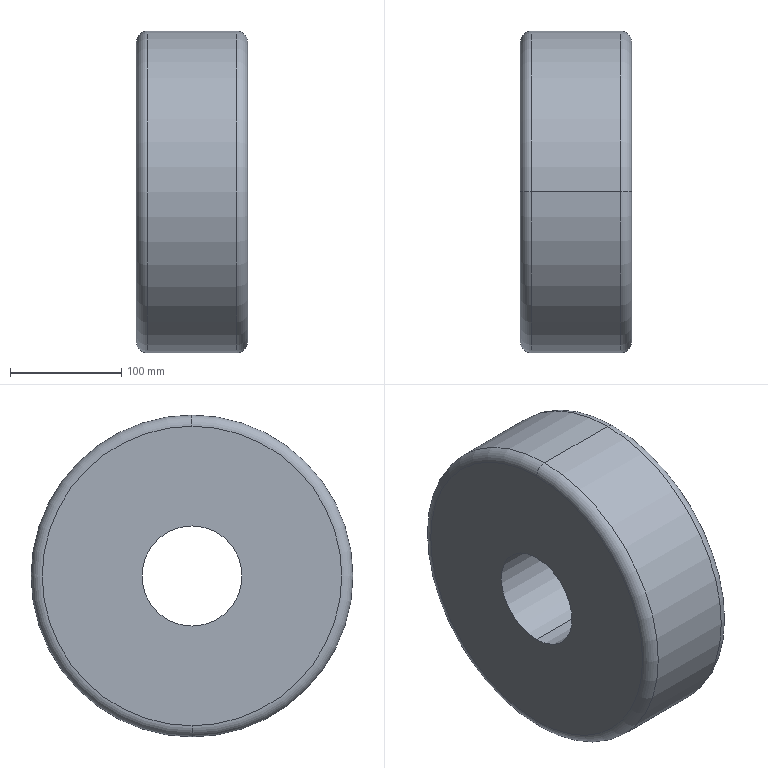Part | SolidWorks | features Fillet 1, Revolution 1 | 1 solid | 10 faces | box 100 x 289 x 289 mm | volume 5885186 mm3 | torus 4 | cylinder 4 | plane 2 | commonest cylinder face diameters 90 x2 289 x2
STEP:
#1=CARTESIAN_POINT('',(-50.,0.,134.5));
#2=VERTEX_POINT('',#1);
#3=CARTESIAN_POINT('',(-50.,0.,-134.5));
#4=VERTEX_POINT('',#3);
#5=CARTESIAN_POINT('',(-50.,0.,0.));
#6=DIRECTION('',(-1.,0.,0.));
#7=DIRECTION('',(0.,0.,-1.));
#8=AXIS2_PLACEMENT_3D('',#5,#6,#7);
#9=CIRCLE('',#8,134.5);
#10=EDGE_CURVE('',#2,#4,#9,.T.);
#11=ORIENTED_EDGE('',*,*,#10,.F.);
#12=CARTESIAN_POINT('',(-40.,0.,144.5));
#13=VERTEX_POINT('',#12);
#14=CARTESIAN_POINT('',(-40.,0.,134.5));
#15=DIRECTION('',(0.,1.,0.));
#16=DIRECTION('',(0.,0.,1.));
#17=AXIS2_PLACEMENT_3D('',#14,#15,#16);
#18=CIRCLE('',#17,10.);
#19=EDGE_CURVE('',#2,#13,#18,.T.);
#20=ORIENTED_EDGE('',*,*,#19,.T.);
#21=CARTESIAN_POINT('',(-40.,0.,-144.5));
#22=VERTEX_POINT('',#21);
#23=CARTESIAN_POINT('',(-40.,0.,0.));
#24=DIRECTION('',(1.,0.,0.));
#25=DIRECTION('',(0.,0.,-1.));
#26=AXIS2_PLACEMENT_3D('',#23,#24,#25);
#27=CIRCLE('',#26,144.5);
#28=EDGE_CURVE('',#22,#13,#27,.T.);
#29=ORIENTED_EDGE('',*,*,#28,.F.);
#30=CARTESIAN_POINT('',(-40.,0.,-134.5));
#31=DIRECTION('',(0.,-1.,0.));
#32=DIRECTION('',(0.,0.,-1.));
#33=AXIS2_PLACEMENT_3D('',#30,#31,#32);
#34=CIRCLE('',#33,10.);
#35=EDGE_CURVE('',#4,#22,#34,.T.);
#36=ORIENTED_EDGE('',*,*,#35,.F.);
#37=EDGE_LOOP('',(#11,#20,#29,#36));
#38=FACE_OUTER_BOUND('',#37,.T.);
#39=CARTESIAN_POINT('',(-40.,0.,0.));
#40=DIRECTION('',(1.,0.,0.));
#41=DIRECTION('',(0.,0.,-1.));
#42=AXIS2_PLACEMENT_3D('',#39,#40,#41);
#43=TOROIDAL_SURFACE('',#42,134.5,10.);
#44=ADVANCED_FACE('',(#38),#43,.T.);
#45=CARTESIAN_POINT('',(50.,0.,-134.5));
#46=VERTEX_POINT('',#45);
#47=CARTESIAN_POINT('',(50.,0.,134.5));
#48=VERTEX_POINT('',#47);
#49=CARTESIAN_POINT('',(50.,0.,0.));
#50=DIRECTION('',(1.,0.,0.));
#51=DIRECTION('',(0.,0.,1.));
#52=AXIS2_PLACEMENT_3D('',#49,#50,#51);
#53=CIRCLE('',#52,134.5);
#54=EDGE_CURVE('',#46,#48,#53,.T.);
#55=ORIENTED_EDGE('',*,*,#54,.F.);
#56=CARTESIAN_POINT('',(40.,0.,-144.5));
#57=VERTEX_POINT('',#56);
#58=CARTESIAN_POINT('',(40.,0.,-134.5));
#59=DIRECTION('',(0.,1.,0.));
#60=DIRECTION('',(0.,0.,1.));
#61=AXIS2_PLACEMENT_3D('',#58,#59,#60);
#62=CIRCLE('',#61,10.);
#63=EDGE_CURVE('',#46,#57,#62,.T.);
#64=ORIENTED_EDGE('',*,*,#63,.T.);
#65=CARTESIAN_POINT('',(40.,0.,144.5));
#66=VERTEX_POINT('',#65);
#67=CARTESIAN_POINT('',(40.,0.,0.));
#68=DIRECTION('',(-1.,0.,0.));
#69=DIRECTION('',(0.,0.,1.));
#70=AXIS2_PLACEMENT_3D('',#67,#68,#69);
#71=CIRCLE('',#70,144.5);
#72=EDGE_CURVE('',#66,#57,#71,.T.);
#73=ORIENTED_EDGE('',*,*,#72,.F.);
#74=CARTESIAN_POINT('',(40.,0.,134.5));
#75=DIRECTION('',(0.,-1.,0.));
#76=DIRECTION('',(0.,0.,-1.));
#77=AXIS2_PLACEMENT_3D('',#74,#75,#76);
#78=CIRCLE('',#77,10.);
#79=EDGE_CURVE('',#48,#66,#78,.T.);
#80=ORIENTED_EDGE('',*,*,#79,.F.);
#81=EDGE_LOOP('',(#55,#64,#73,#80));
#82=FACE_OUTER_BOUND('',#81,.T.);
#83=CARTESIAN_POINT('',(40.,0.,0.));
#84=DIRECTION('',(-1.,0.,0.));
#85=DIRECTION('',(0.,0.,1.));
#86=AXIS2_PLACEMENT_3D('',#83,#84,#85);
#87=TOROIDAL_SURFACE('',#86,134.5,10.);
#88=ADVANCED_FACE('',(#82),#87,.T.);
#89=ORIENTED_EDGE('',*,*,#72,.T.);
#90=CARTESIAN_POINT('',(-106.18,0.,-144.5));
#91=DIRECTION('',(-1.,0.,0.));
#92=VECTOR('',#91,1000.);
#93=LINE('',#90,#92);
#94=EDGE_CURVE('',#57,#22,#93,.T.);
#95=ORIENTED_EDGE('',*,*,#94,.T.);
#96=ORIENTED_EDGE('',*,*,#28,.T.);
#97=CARTESIAN_POINT('',(-106.18,0.,144.5));
#98=DIRECTION('',(-1.,0.,0.));
#99=VECTOR('',#98,1000.);
#100=LINE('',#97,#99);
#101=EDGE_CURVE('',#66,#13,#100,.T.);
#102=ORIENTED_EDGE('',*,*,#101,.F.);
#103=EDGE_LOOP('',(#89,#95,#96,#102));
#104=FACE_OUTER_BOUND('',#103,.T.);
#105=CARTESIAN_POINT('',(-106.18,0.,0.));
#106=DIRECTION('',(-1.,0.,0.));
#107=DIRECTION('',(0.,0.,1.));
#108=AXIS2_PLACEMENT_3D('',#105,#106,#107);
#109=CYLINDRICAL_SURFACE('',#108,144.5);
#110=ADVANCED_FACE('',(#104),#109,.T.);
#111=CARTESIAN_POINT('',(50.,0.,-45.));
#112=VERTEX_POINT('',#111);
#113=CARTESIAN_POINT('',(50.,0.,45.));
#114=VERTEX_POINT('',#113);
#115=CARTESIAN_POINT('',(50.,0.,0.));
#116=DIRECTION('',(-1.,0.,0.));
#117=DIRECTION('',(0.,0.,1.));
#118=AXIS2_PLACEMENT_3D('',#115,#116,#117);
#119=CIRCLE('',#118,45.);
#120=EDGE_CURVE('',#112,#114,#119,.T.);
#121=ORIENTED_EDGE('',*,*,#120,.F.);
#122=CARTESIAN_POINT('',(-50.,0.,-45.));
#123=VERTEX_POINT('',#122);
#124=CARTESIAN_POINT('',(-106.18,0.,-45.));
#125=DIRECTION('',(-1.,0.,0.));
#126=VECTOR('',#125,1000.);
#127=LINE('',#124,#126);
#128=EDGE_CURVE('',#112,#123,#127,.T.);
#129=ORIENTED_EDGE('',*,*,#128,.T.);
#130=CARTESIAN_POINT('',(-50.,0.,45.));
#131=VERTEX_POINT('',#130);
#132=CARTESIAN_POINT('',(-50.,0.,0.));
#133=DIRECTION('',(-1.,0.,0.));
#134=DIRECTION('',(0.,0.,1.));
#135=AXIS2_PLACEMENT_3D('',#132,#133,#134);
#136=CIRCLE('',#135,45.);
#137=EDGE_CURVE('',#123,#131,#136,.T.);
#138=ORIENTED_EDGE('',*,*,#137,.T.);
#139=CARTESIAN_POINT('',(-106.18,0.,45.));
#140=DIRECTION('',(-1.,0.,0.));
#141=VECTOR('',#140,1000.);
#142=LINE('',#139,#141);
#143=EDGE_CURVE('',#114,#131,#142,.T.);
#144=ORIENTED_EDGE('',*,*,#143,.F.);
#145=EDGE_LOOP('',(#121,#129,#138,#144));
#146=FACE_OUTER_BOUND('',#145,.T.);
#147=CARTESIAN_POINT('',(-106.18,0.,0.));
#148=DIRECTION('',(-1.,0.,0.));
#149=DIRECTION('',(0.,0.,1.));
#150=AXIS2_PLACEMENT_3D('',#147,#148,#149);
#151=CYLINDRICAL_SURFACE('',#150,45.);
#152=ADVANCED_FACE('',(#146),#151,.F.);
#153=CARTESIAN_POINT('',(50.,0.,0.));
#154=DIRECTION('',(1.,0.,0.));
#155=DIRECTION('',(0.,0.,1.));
#156=AXIS2_PLACEMENT_3D('',#153,#154,#155);
#157=CIRCLE('',#156,134.5);
#158=EDGE_CURVE('',#48,#46,#157,.T.);
#159=ORIENTED_EDGE('',*,*,#158,.T.);
#160=ORIENTED_EDGE('',*,*,#54,.T.);
#161=EDGE_LOOP('',(#159,#160));
#162=FACE_OUTER_BOUND('',#161,.T.);
#163=CARTESIAN_POINT('',(50.,0.,0.));
#164=DIRECTION('',(-1.,0.,0.));
#165=DIRECTION('',(0.,0.,1.));
#166=AXIS2_PLACEMENT_3D('',#163,#164,#165);
#167=CIRCLE('',#166,45.);
#168=EDGE_CURVE('',#114,#112,#167,.T.);
#169=ORIENTED_EDGE('',*,*,#168,.T.);
#170=ORIENTED_EDGE('',*,*,#120,.T.);
#171=EDGE_LOOP('',(#169,#170));
#172=FACE_BOUND('',#171,.T.);
#173=CARTESIAN_POINT('',(50.,45.,0.));
#174=DIRECTION('',(-1.,0.,0.));
#175=DIRECTION('',(0.,0.,1.));
#176=AXIS2_PLACEMENT_3D('',#173,#174,#175);
#177=PLANE('',#176);
#178=ADVANCED_FACE('',(#162,#172),#177,.F.);
#179=ORIENTED_EDGE('',*,*,#128,.F.);
#180=ORIENTED_EDGE('',*,*,#168,.F.);
#181=ORIENTED_EDGE('',*,*,#143,.T.);
#182=CARTESIAN_POINT('',(-50.,0.,0.));
#183=DIRECTION('',(-1.,0.,0.));
#184=DIRECTION('',(0.,0.,1.));
#185=AXIS2_PLACEMENT_3D('',#182,#183,#184);
#186=CIRCLE('',#185,45.);
#187=EDGE_CURVE('',#131,#123,#186,.T.);
#188=ORIENTED_EDGE('',*,*,#187,.T.);
#189=EDGE_LOOP('',(#179,#180,#181,#188));
#190=FACE_OUTER_BOUND('',#189,.T.);
#191=CARTESIAN_POINT('',(-106.18,0.,0.));
#192=DIRECTION('',(-1.,0.,0.));
#193=DIRECTION('',(0.,0.,1.));
#194=AXIS2_PLACEMENT_3D('',#191,#192,#193);
#195=CYLINDRICAL_SURFACE('',#194,45.);
#196=ADVANCED_FACE('',(#190),#195,.F.);
#197=CARTESIAN_POINT('',(-50.,0.,0.));
#198=DIRECTION('',(-1.,0.,0.));
#199=DIRECTION('',(0.,0.,-1.));
#200=AXIS2_PLACEMENT_3D('',#197,#198,#199);
#201=CIRCLE('',#200,134.5);
#202=EDGE_CURVE('',#4,#2,#201,.T.);
#203=ORIENTED_EDGE('',*,*,#202,.T.);
#204=ORIENTED_EDGE('',*,*,#10,.T.);
#205=EDGE_LOOP('',(#203,#204));
#206=FACE_OUTER_BOUND('',#205,.T.);
#207=ORIENTED_EDGE('',*,*,#187,.F.);
#208=ORIENTED_EDGE('',*,*,#137,.F.);
#209=EDGE_LOOP('',(#207,#208));
#210=FACE_BOUND('',#209,.T.);
#211=CARTESIAN_POINT('',(-50.,45.,0.));
#212=DIRECTION('',(1.,0.,0.));
#213=DIRECTION('',(0.,0.,-1.));
#214=AXIS2_PLACEMENT_3D('',#211,#212,#213);
#215=PLANE('',#214);
#216=ADVANCED_FACE('',(#206,#210),#215,.F.);
#217=ORIENTED_EDGE('',*,*,#94,.F.);
#218=CARTESIAN_POINT('',(40.,0.,0.));
#219=DIRECTION('',(-1.,0.,0.));
#220=DIRECTION('',(0.,0.,1.));
#221=AXIS2_PLACEMENT_3D('',#218,#219,#220);
#222=CIRCLE('',#221,144.5);
#223=EDGE_CURVE('',#57,#66,#222,.T.);
#224=ORIENTED_EDGE('',*,*,#223,.T.);
#225=ORIENTED_EDGE('',*,*,#101,.T.);
#226=CARTESIAN_POINT('',(-40.,0.,0.));
#227=DIRECTION('',(1.,0.,0.));
#228=DIRECTION('',(0.,0.,-1.));
#229=AXIS2_PLACEMENT_3D('',#226,#227,#228);
#230=CIRCLE('',#229,144.5);
#231=EDGE_CURVE('',#13,#22,#230,.T.);
#232=ORIENTED_EDGE('',*,*,#231,.T.);
#233=EDGE_LOOP('',(#217,#224,#225,#232));
#234=FACE_OUTER_BOUND('',#233,.T.);
#235=CARTESIAN_POINT('',(-106.18,0.,0.));
#236=DIRECTION('',(-1.,0.,0.));
#237=DIRECTION('',(0.,0.,1.));
#238=AXIS2_PLACEMENT_3D('',#235,#236,#237);
#239=CYLINDRICAL_SURFACE('',#238,144.5);
#240=ADVANCED_FACE('',(#234),#239,.T.);
#241=ORIENTED_EDGE('',*,*,#63,.F.);
#242=ORIENTED_EDGE('',*,*,#158,.F.);
#243=ORIENTED_EDGE('',*,*,#79,.T.);
#244=ORIENTED_EDGE('',*,*,#223,.F.);
#245=EDGE_LOOP('',(#241,#242,#243,#244));
#246=FACE_OUTER_BOUND('',#245,.T.);
#247=CARTESIAN_POINT('',(40.,0.,0.));
#248=DIRECTION('',(-1.,0.,0.));
#249=DIRECTION('',(0.,0.,1.));
#250=AXIS2_PLACEMENT_3D('',#247,#248,#249);
#251=TOROIDAL_SURFACE('',#250,134.5,10.);
#252=ADVANCED_FACE('',(#246),#251,.T.);
#253=ORIENTED_EDGE('',*,*,#19,.F.);
#254=ORIENTED_EDGE('',*,*,#202,.F.);
#255=ORIENTED_EDGE('',*,*,#35,.T.);
#256=ORIENTED_EDGE('',*,*,#231,.F.);
#257=EDGE_LOOP('',(#253,#254,#255,#256));
#258=FACE_OUTER_BOUND('',#257,.T.);
#259=CARTESIAN_POINT('',(-40.,0.,0.));
#260=DIRECTION('',(1.,0.,0.));
#261=DIRECTION('',(0.,0.,-1.));
#262=AXIS2_PLACEMENT_3D('',#259,#260,#261);
#263=TOROIDAL_SURFACE('',#262,134.5,10.);
#264=ADVANCED_FACE('',(#258),#263,.T.);
#265=CLOSED_SHELL('',(#44,#88,#110,#152,#178,#196,#216,#240,#252,#264));
#266=MANIFOLD_SOLID_BREP('',#265);
#267=CARTESIAN_POINT('',(0.,0.,0.));
#268=DIRECTION('',(0.,0.,1.));
#269=DIRECTION('',(1.,0.,0.));
#270=AXIS2_PLACEMENT_3D('',#267,#268,#269);
#271=(LENGTH_UNIT()NAMED_UNIT(*)SI_UNIT(.MILLI.,.METRE.));
#272=UNCERTAINTY_MEASURE_WITH_UNIT(LENGTH_MEASURE(0.00001),#271,'','');
#273=(NAMED_UNIT(*)PLANE_ANGLE_UNIT()SI_UNIT($,.RADIAN.));
#274=(NAMED_UNIT(*)SI_UNIT($,.STERADIAN.)SOLID_ANGLE_UNIT());
#275=(GEOMETRIC_REPRESENTATION_CONTEXT(3)GLOBAL_UNCERTAINTY_ASSIGNED_CONTEXT((#272))GLOBAL_UNIT_ASSIGNED_CONTEXT((#271,#273,#274))REPRESENTATION_CONTEXT('',''));
#276=ADVANCED_BREP_SHAPE_REPRESENTATION('',(#266,#270),#275);